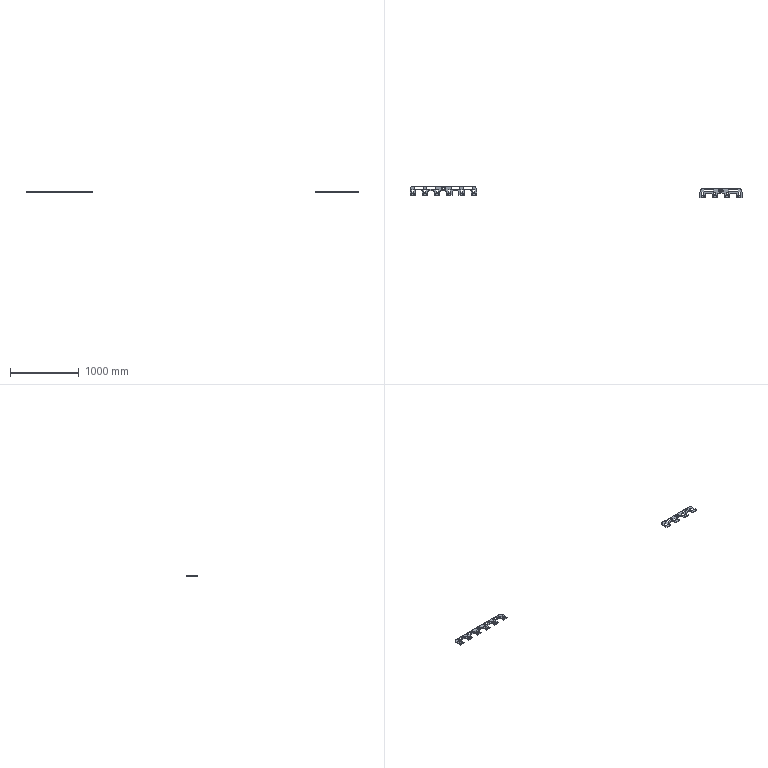NC program | NX | posted with a generic post | part box 4825 x 168.213 x 13 mm
Lines 138 to 1364 of 14244:
(ZLEVEL_PROFILE_COPY_3 , TOOL : D10)
N256 T10 M6
N258 G54
N260 G17 G0 G90 X8.032 Y52.717 S9500 M3
N262 G43 Z30. H10
N264 Z1.5
N266 G94 G1 X8.068 Y52.76 Z1.497 F1000.
N268 X10.015 Y54.925 Z1.344
N270 X12.075 Y56.985 Z1.192
N272 X14.24 Y58.932 Z1.039
N274 X16.505 Y60.763 Z0.887
N276 X18.864 Y62.471 Z0.734
N278 X21.309 Y64.053 Z0.581
N280 X23.835 Y65.503 Z0.429
N282 X26.434 Y66.817 Z0.276
N284 X29.098 Y67.992 Z0.123
N286 X31.821 Y69.025 Z-0.029
N288 X34.595 Y69.913 Z-0.182
N290 X37.412 Y70.653 Z-0.334
N292 X40.264 Y71.243 Z-0.487
N294 X43.143 Y71.682 Z-0.64
N296 X46.041 Y71.968 Z-0.792
N298 X48.95 Y72.1 Z-0.945
N300 X50. Z-1.
N302 X916.8 F3500.
N304 G2 X971.9 Y17. R55.1
N306 G1 Y-67.
N308 G2 X966.8 Y-72.1 R5.1
N310 G1 X889.
N312 G2 X883.9 Y-67. R5.1
N314 G1 Y-5.
N316 G3 X869. Y9.9 R14.9
N318 G1 X809.
N320 G3 X794.1 Y-5. R14.9
N322 G1 Y-67.
N324 G2 X789. Y-72.1 R5.1
N326 G1 X711.2
N328 G2 X706.1 Y-67. R5.1
N330 G1 Y-20.95
N332 G3 X691.2 Y-6.05 R14.9
N334 G1 X631.2
N336 G3 X616.3 Y-20.95 R14.9
N338 G1 Y-67.
N340 G2 X611.2 Y-72.1 R5.1
N342 G1 X533.4
N344 G2 X528.3 Y-67. R5.1
N346 G1 Y-20.95
N348 G3 X513.4 Y-6.05 R14.9
N350 G1 X453.4
N352 G3 X438.5 Y-20.95 R14.9
N354 G1 Y-67.
N356 G2 X433.4 Y-72.1 R5.1
N358 G1 X355.6
N360 G2 X350.5 Y-67. R5.1
N362 G1 Y-20.95
N364 G3 X335.6 Y-6.05 R14.9
N366 G1 X275.6
N368 G3 X260.7 Y-20.95 R14.9
N370 G1 Y-67.
N372 G2 X255.6 Y-72.1 R5.1
N374 G1 X177.8
N376 G2 X172.7 Y-67. R5.1
N378 G1 Y-5.
N380 G3 X157.8 Y9.9 R14.9
N382 G1 X97.8
N384 G3 X82.9 Y-5. R14.9
N386 G1 Y-67.
N388 G2 X77.8 Y-72.1 R5.1
N390 G1 X0.
N392 G2 X-5.1 Y-67. R5.1
N394 G1 Y17.
N396 G2 X50. Y72.1 R55.1
N398 G1 X107.29 Z-2.
N400 X916.8
N402 G2 X971.9 Y17. R55.1
N404 G1 Y-67.
N406 G2 X966.8 Y-72.1 R5.1
N408 G1 X889.
N410 G2 X883.9 Y-67. R5.1
N412 G1 Y-5.
N414 G3 X869. Y9.9 R14.9
N416 G1 X809.
N418 G3 X794.1 Y-5. R14.9
N420 G1 Y-67.
N422 G2 X789. Y-72.1 R5.1
N424 G1 X711.2
N426 G2 X706.1 Y-67. R5.1
N428 G1 Y-20.95
N430 G3 X691.2 Y-6.05 R14.9
N432 G1 X631.2
N434 G3 X616.3 Y-20.95 R14.9
N436 G1 Y-67.
N438 G2 X611.2 Y-72.1 R5.1
N440 G1 X533.4
N442 G2 X528.3 Y-67. R5.1
N444 G1 Y-20.95
N446 G3 X513.4 Y-6.05 R14.9
N448 G1 X453.4
N450 G3 X438.5 Y-20.95 R14.9
N452 G1 Y-67.
N454 G2 X433.4 Y-72.1 R5.1
N456 G1 X355.6
N458 G2 X350.5 Y-67. R5.1
N460 G1 Y-20.95
N462 G3 X335.6 Y-6.05 R14.9
N464 G1 X275.6
N466 G3 X260.7 Y-20.95 R14.9
N468 G1 Y-67.
N470 G2 X255.6 Y-72.1 R5.1
N472 G1 X177.8
N474 G2 X172.7 Y-67. R5.1
N476 G1 Y-5.
N478 G3 X157.8 Y9.9 R14.9
N480 G1 X97.8
N482 G3 X82.9 Y-5. R14.9
N484 G1 Y-67.
N486 G2 X77.8 Y-72.1 R5.1
N488 G1 X0.
N490 G2 X-5.1 Y-67. R5.1
N492 G1 Y17.
N494 G2 X50. Y72.1 R55.1
N496 G1 X107.29 Z-3.
N498 X916.8
N500 G2 X971.9 Y17. R55.1
N502 G1 Y-67.
N504 G2 X966.8 Y-72.1 R5.1
N506 G1 X889.
N508 G2 X883.9 Y-67. R5.1
N510 G1 Y-5.
N512 G3 X869. Y9.9 R14.9
N514 G1 X809.
N516 G3 X794.1 Y-5. R14.9
N518 G1 Y-67.
N520 G2 X789. Y-72.1 R5.1
N522 G1 X711.2
N524 G2 X706.1 Y-67. R5.1
N526 G1 Y-20.95
N528 G3 X691.2 Y-6.05 R14.9
N530 G1 X631.2
N532 G3 X616.3 Y-20.95 R14.9
N534 G1 Y-67.
N536 G2 X611.2 Y-72.1 R5.1
N538 G1 X533.4
N540 G2 X528.3 Y-67. R5.1
N542 G1 Y-20.95
N544 G3 X513.4 Y-6.05 R14.9
N546 G1 X453.4
N548 G3 X438.5 Y-20.95 R14.9
N550 G1 Y-67.
N552 G2 X433.4 Y-72.1 R5.1
N554 G1 X355.6
N556 G2 X350.5 Y-67. R5.1
N558 G1 Y-20.95
N560 G3 X335.6 Y-6.05 R14.9
N562 G1 X275.6
N564 G3 X260.7 Y-20.95 R14.9
N566 G1 Y-67.
N568 G2 X255.6 Y-72.1 R5.1
N570 G1 X177.8
N572 G2 X172.7 Y-67. R5.1
N574 G1 Y-5.
N576 G3 X157.8 Y9.9 R14.9
N578 G1 X97.8
N580 G3 X82.9 Y-5. R14.9
N582 G1 Y-67.
N584 G2 X77.8 Y-72.1 R5.1
N586 G1 X0.
N588 G2 X-5.1 Y-67. R5.1
N590 G1 Y17.
N592 G2 X50. Y72.1 R55.1
N594 G1 X95.832 Z-3.8
N596 X916.8
N598 G2 X971.9 Y17. R55.1
N600 G1 Y-67.
N602 G2 X966.8 Y-72.1 R5.1
N604 G1 X889.
N606 G2 X883.9 Y-67. R5.1
N608 G1 Y-5.
N610 G3 X869. Y9.9 R14.9
N612 G1 X809.
N614 G3 X794.1 Y-5. R14.9
N616 G1 Y-67.
N618 G2 X789. Y-72.1 R5.1
N620 G1 X711.2
N622 G2 X706.1 Y-67. R5.1
N624 G1 Y-20.95
N626 G3 X691.2 Y-6.05 R14.9
N628 G1 X631.2
N630 G3 X616.3 Y-20.95 R14.9
N632 G1 Y-67.
N634 G2 X611.2 Y-72.1 R5.1
N636 G1 X533.4
N638 G2 X528.3 Y-67. R5.1
N640 G1 Y-20.95
N642 G3 X513.4 Y-6.05 R14.9
N644 G1 X453.4
N646 G3 X438.5 Y-20.95 R14.9
N648 G1 Y-67.
N650 G2 X433.4 Y-72.1 R5.1
N652 G1 X355.6
N654 G2 X350.5 Y-67. R5.1
N656 G1 Y-20.95
N658 G3 X335.6 Y-6.05 R14.9
N660 G1 X275.6
N662 G3 X260.7 Y-20.95 R14.9
N664 G1 Y-67.
N666 G2 X255.6 Y-72.1 R5.1
N668 G1 X177.8
N670 G2 X172.7 Y-67. R5.1
N672 G1 Y-5.
N674 G3 X157.8 Y9.9 R14.9
N676 G1 X97.8
N678 G3 X82.9 Y-5. R14.9
N680 G1 Y-67.
N682 G2 X77.8 Y-72.1 R5.1
N684 G1 X0.
N686 G2 X-5.1 Y-67. R5.1
N688 G1 Y17.
N690 G2 X50. Y72.1 R55.1
N692 G1 X95.832 Z-4.6
N694 X916.8
N696 G2 X971.9 Y17. R55.1
N698 G1 Y-67.
N700 G2 X966.8 Y-72.1 R5.1
N702 G1 X889.
N704 G2 X883.9 Y-67. R5.1
N706 G1 Y-5.
N708 G3 X869. Y9.9 R14.9
N710 G1 X809.
N712 G3 X794.1 Y-5. R14.9
N714 G1 Y-67.
N716 G2 X789. Y-72.1 R5.1
N718 G1 X711.2
N720 G2 X706.1 Y-67. R5.1
N722 G1 Y-20.95
N724 G3 X691.2 Y-6.05 R14.9
N726 G1 X631.2
N728 G3 X616.3 Y-20.95 R14.9
N730 G1 Y-67.
N732 G2 X611.2 Y-72.1 R5.1
N734 G1 X533.4
N736 G2 X528.3 Y-67. R5.1
N738 G1 Y-20.95
N740 G3 X513.4 Y-6.05 R14.9
N742 G1 X453.4
N744 G3 X438.5 Y-20.95 R14.9
N746 G1 Y-67.
N748 G2 X433.4 Y-72.1 R5.1
N750 G1 X355.6
N752 G2 X350.5 Y-67. R5.1
N754 G1 Y-20.95
N756 G3 X335.6 Y-6.05 R14.9
N758 G1 X275.6
N760 G3 X260.7 Y-20.95 R14.9
N762 G1 Y-67.
N764 G2 X255.6 Y-72.1 R5.1
N766 G1 X177.8
N768 G2 X172.7 Y-67. R5.1
N770 G1 Y-5.
N772 G3 X157.8 Y9.9 R14.9
N774 G1 X97.8
N776 G3 X82.9 Y-5. R14.9
N778 G1 Y-67.
N780 G2 X77.8 Y-72.1 R5.1
N782 G1 X0.
N784 G2 X-5.1 Y-67. R5.1
N786 G1 Y17.
N788 G2 X50. Y72.1 R55.1
N790 G1 X105.858 Z-5.575
N792 X916.8
N794 G2 X971.9 Y17. R55.1
N796 G1 Y-67.
N798 G2 X966.8 Y-72.1 R5.1
N800 G1 X889.
N802 G2 X883.9 Y-67. R5.1
N804 G1 Y-5.
N806 G3 X869. Y9.9 R14.9
N808 G1 X809.
N810 G3 X794.1 Y-5. R14.9
N812 G1 Y-67.
N814 G2 X789. Y-72.1 R5.1
N816 G1 X711.2
N818 G2 X706.1 Y-67. R5.1
N820 G1 Y-20.95
N822 G3 X691.2 Y-6.05 R14.9
N824 G1 X631.2
N826 G3 X616.3 Y-20.95 R14.9
N828 G1 Y-67.
N830 G2 X611.2 Y-72.1 R5.1
N832 G1 X533.4
N834 G2 X528.3 Y-67. R5.1
N836 G1 Y-20.95
N838 G3 X513.4 Y-6.05 R14.9
N840 G1 X453.4
N842 G3 X438.5 Y-20.95 R14.9
N844 G1 Y-67.
N846 G2 X433.4 Y-72.1 R5.1
N848 G1 X355.6
N850 G2 X350.5 Y-67. R5.1
N852 G1 Y-20.95
N854 G3 X335.6 Y-6.05 R14.9
N856 G1 X275.6
N858 G3 X260.7 Y-20.95 R14.9
N860 G1 Y-67.
N862 G2 X255.6 Y-72.1 R5.1
N864 G1 X177.8
N866 G2 X172.7 Y-67. R5.1
N868 G1 Y-5.
N870 G3 X157.8 Y9.9 R14.9
N872 G1 X97.8
N874 G3 X82.9 Y-5. R14.9
N876 G1 Y-67.
N878 G2 X77.8 Y-72.1 R5.1
N880 G1 X0.
N882 G2 X-5.1 Y-67. R5.1
N884 G1 Y17.
N886 G2 X50. Y72.1 R55.1
N888 G1 X105.858 Z-6.55
N890 X916.8
N892 G2 X971.9 Y17. R55.1
N894 G1 Y-67.
N896 G2 X966.8 Y-72.1 R5.1
N898 G1 X889.
N900 G2 X883.9 Y-67. R5.1
N902 G1 Y-5.
N904 G3 X869. Y9.9 R14.9
N906 G1 X809.
N908 G3 X794.1 Y-5. R14.9
N910 G1 Y-67.
N912 G2 X789. Y-72.1 R5.1
N914 G1 X711.2
N916 G2 X706.1 Y-67. R5.1
N918 G1 Y-20.95
N920 G3 X691.2 Y-6.05 R14.9
N922 G1 X631.2
N924 G3 X616.3 Y-20.95 R14.9
N926 G1 Y-67.
N928 G2 X611.2 Y-72.1 R5.1
N930 G1 X533.4
N932 G2 X528.3 Y-67. R5.1
N934 G1 Y-20.95
N936 G3 X513.4 Y-6.05 R14.9
N938 G1 X453.4
N940 G3 X438.5 Y-20.95 R14.9
N942 G1 Y-67.
N944 G2 X433.4 Y-72.1 R5.1
N946 G1 X355.6
N948 G2 X350.5 Y-67. R5.1
N950 G1 Y-20.95
N952 G3 X335.6 Y-6.05 R14.9
N954 G1 X275.6
N956 G3 X260.7 Y-20.95 R14.9
N958 G1 Y-67.
N960 G2 X255.6 Y-72.1 R5.1
N962 G1 X177.8
N964 G2 X172.7 Y-67. R5.1
N966 G1 Y-5.
N968 G3 X157.8 Y9.9 R14.9
N970 G1 X97.8
N972 G3 X82.9 Y-5. R14.9
N974 G1 Y-67.
N976 G2 X77.8 Y-72.1 R5.1
N978 G1 X0.
N980 G2 X-5.1 Y-67. R5.1
N982 G1 Y17.
N984 G2 X50. Y72.1 R55.1
N986 G1 X105.858 Z-7.525
N988 X916.8
N990 G2 X971.9 Y17. R55.1
N992 G1 Y-67.
N994 G2 X966.8 Y-72.1 R5.1
N996 G1 X889.
N998 G2 X883.9 Y-67. R5.1
N1000 G1 Y-5.
N1002 G3 X869. Y9.9 R14.9
N1004 G1 X809.
N1006 G3 X794.1 Y-5. R14.9
N1008 G1 Y-67.
N1010 G2 X789. Y-72.1 R5.1
N1012 G1 X711.2
N1014 G2 X706.1 Y-67. R5.1
N1016 G1 Y-20.95
N1018 G3 X691.2 Y-6.05 R14.9
N1020 G1 X631.2
N1022 G3 X616.3 Y-20.95 R14.9
N1024 G1 Y-67.
N1026 G2 X611.2 Y-72.1 R5.1
N1028 G1 X533.4
N1030 G2 X528.3 Y-67. R5.1
N1032 G1 Y-20.95
N1034 G3 X513.4 Y-6.05 R14.9
N1036 G1 X453.4
N1038 G3 X438.5 Y-20.95 R14.9
N1040 G1 Y-67.
N1042 G2 X433.4 Y-72.1 R5.1
N1044 G1 X355.6
N1046 G2 X350.5 Y-67. R5.1
N1048 G1 Y-20.95
N1050 G3 X335.6 Y-6.05 R14.9
N1052 G1 X275.6
N1054 G3 X260.7 Y-20.95 R14.9
N1056 G1 Y-67.
N1058 G2 X255.6 Y-72.1 R5.1
N1060 G1 X177.8
N1062 G2 X172.7 Y-67. R5.1
N1064 G1 Y-5.
N1066 G3 X157.8 Y9.9 R14.9
N1068 G1 X97.8
N1070 G3 X82.9 Y-5. R14.9
N1072 G1 Y-67.
N1074 G2 X77.8 Y-72.1 R5.1
N1076 G1 X0.
N1078 G2 X-5.1 Y-67. R5.1
N1080 G1 Y17.
N1082 G2 X50. Y72.1 R55.1
N1084 G1 X105.858 Z-8.5
N1086 X916.8
N1088 G2 X971.9 Y17. R55.1
N1090 G1 Y-67.
N1092 G2 X966.8 Y-72.1 R5.1
N1094 G1 X889.
N1096 G2 X883.9 Y-67. R5.1
N1098 G1 Y-5.
N1100 G3 X869. Y9.9 R14.9
N1102 G1 X809.
N1104 G3 X794.1 Y-5. R14.9
N1106 G1 Y-67.
N1108 G2 X789. Y-72.1 R5.1
N1110 G1 X711.2
N1112 G2 X706.1 Y-67. R5.1
N1114 G1 Y-20.95
N1116 G3 X691.2 Y-6.05 R14.9
N1118 G1 X631.2
N1120 G3 X616.3 Y-20.95 R14.9
N1122 G1 Y-67.
N1124 G2 X611.2 Y-72.1 R5.1
N1126 G1 X533.4
N1128 G2 X528.3 Y-67. R5.1
N1130 G1 Y-20.95
N1132 G3 X513.4 Y-6.05 R14.9
N1134 G1 X453.4
N1136 G3 X438.5 Y-20.95 R14.9
N1138 G1 Y-67.
N1140 G2 X433.4 Y-72.1 R5.1
N1142 G1 X355.6
N1144 G2 X350.5 Y-67. R5.1
N1146 G1 Y-20.95
N1148 G3 X335.6 Y-6.05 R14.9
N1150 G1 X275.6
N1152 G3 X260.7 Y-20.95 R14.9
N1154 G1 Y-67.
N1156 G2 X255.6 Y-72.1 R5.1
N1158 G1 X177.8
N1160 G2 X172.7 Y-67. R5.1
N1162 G1 Y-5.
N1164 G3 X157.8 Y9.9 R14.9
N1166 G1 X97.8
N1168 G3 X82.9 Y-5. R14.9
N1170 G1 Y-67.
N1172 G2 X77.8 Y-72.1 R5.1
N1174 G1 X0.
N1176 G2 X-5.1 Y-67. R5.1
N1178 G1 Y17.
N1180 G2 X50. Y72.1 R55.1
N1182 G1 X105.858 Z-9.475
N1184 X916.8
N1186 G2 X971.9 Y17. R55.1
N1188 G1 Y-67.
N1190 G2 X966.8 Y-72.1 R5.1
N1192 G1 X889.
N1194 G2 X883.9 Y-67. R5.1
N1196 G1 Y-5.
N1198 G3 X869. Y9.9 R14.9
N1200 G1 X809.
N1202 G3 X794.1 Y-5. R14.9
N1204 G1 Y-67.
N1206 G2 X789. Y-72.1 R5.1
N1208 G1 X711.2
N1210 G2 X706.1 Y-67. R5.1
N1212 G1 Y-20.95
N1214 G3 X691.2 Y-6.05 R14.9
N1216 G1 X631.2
N1218 G3 X616.3 Y-20.95 R14.9
N1220 G1 Y-67.
N1222 G2 X611.2 Y-72.1 R5.1
N1224 G1 X533.4
N1226 G2 X528.3 Y-67. R5.1
N1228 G1 Y-20.95
N1230 G3 X513.4 Y-6.05 R14.9
N1232 G1 X453.4
N1234 G3 X438.5 Y-20.95 R14.9
N1236 G1 Y-67.
N1238 G2 X433.4 Y-72.1 R5.1
N1240 G1 X355.6
N1242 G2 X350.5 Y-67. R5.1
N1244 G1 Y-20.95
N1246 G3 X335.6 Y-6.05 R14.9
N1248 G1 X275.6
N1250 G3 X260.7 Y-20.95 R14.9
N1252 G1 Y-67.
N1254 G2 X255.6 Y-72.1 R5.1
N1256 G1 X177.8
N1258 G2 X172.7 Y-67. R5.1
N1260 G1 Y-5.
N1262 G3 X157.8 Y9.9 R14.9
N1264 G1 X97.8
N1266 G3 X82.9 Y-5. R14.9
N1268 G1 Y-67.
N1270 G2 X77.8 Y-72.1 R5.1
N1272 G1 X0.
N1274 G2 X-5.1 Y-67. R5.1
N1276 G1 Y17.
N1278 G2 X50. Y72.1 R55.1
N1280 G1 X105.858 Z-10.45
N1282 X916.8
N1284 G2 X971.9 Y17. R55.1
N1286 G1 Y-67.
N1288 G2 X966.8 Y-72.1 R5.1
N1290 G1 X889.
N1292 G2 X883.9 Y-67. R5.1
N1294 G1 Y-5.
N1296 G3 X869. Y9.9 R14.9
N1298 G1 X809.
N1300 G3 X794.1 Y-5. R14.9
N1302 G1 Y-67.
N1304 G2 X789. Y-72.1 R5.1
N1306 G1 X711.2
N1308 G2 X706.1 Y-67. R5.1
N1310 G1 Y-20.95
N1312 G3 X691.2 Y-6.05 R14.9
N1314 G1 X631.2
N1316 G3 X616.3 Y-20.95 R14.9
N1318 G1 Y-67.
N1320 G2 X611.2 Y-72.1 R5.1
N1322 G1 X533.4
N1324 G2 X528.3 Y-67. R5.1
N1326 G1 Y-20.95
N1328 G3 X513.4 Y-6.05 R14.9
N1330 G1 X453.4
N1332 G3 X438.5 Y-20.95 R14.9
N1334 G1 Y-67.
N1336 G2 X433.4 Y-72.1 R5.1
N1338 G1 X355.6
N1340 G2 X350.5 Y-67. R5.1
N1342 G1 Y-20.95
N1344 G3 X335.6 Y-6.05 R14.9
N1346 G1 X275.6
N1348 G3 X260.7 Y-20.95 R14.9
N1350 G1 Y-67.
N1352 G2 X255.6 Y-72.1 R5.1
N1354 G1 X177.8
N1356 G2 X172.7 Y-67. R5.1
N1358 G1 Y-5.
N1360 G3 X157.8 Y9.9 R14.9
N1362 G1 X97.8
N1364 G3 X82.9 Y-5. R14.9
N1366 G1 Y-67.
N1368 G2 X77.8 Y-72.1 R5.1
N1370 G1 X0.
N1372 G2 X-5.1 Y-67. R5.1
N1374 G1 Y17.
N1376 G2 X50. Y72.1 R55.1
N1378 G1 X105.858 Z-11.425
N1380 X916.8
N1382 G2 X971.9 Y17. R55.1
N1384 G1 Y-67.
N1386 G2 X966.8 Y-72.1 R5.1
N1388 G1 X889.
N1390 G2 X883.9 Y-67. R5.1
N1392 G1 Y-5.
N1394 G3 X869. Y9.9 R14.9
N1396 G1 X809.
N1398 G3 X794.1 Y-5. R14.9
N1400 G1 Y-67.
N1402 G2 X789. Y-72.1 R5.1
N1404 G1 X711.2
N1406 G2 X706.1 Y-67. R5.1
N1408 G1 Y-20.95
N1410 G3 X691.2 Y-6.05 R14.9
N1412 G1 X631.2
N1414 G3 X616.3 Y-20.95 R14.9
N1416 G1 Y-67.
N1418 G2 X611.2 Y-72.1 R5.1
N1420 G1 X533.4
N1422 G2 X528.3 Y-67. R5.1
N1424 G1 Y-20.95
N1426 G3 X513.4 Y-6.05 R14.9
N1428 G1 X453.4
N1430 G3 X438.5 Y-20.95 R14.9
N1432 G1 Y-67.
N1434 G2 X433.4 Y-72.1 R5.1
N1436 G1 X355.6
N1438 G2 X350.5 Y-67. R5.1
N1440 G1 Y-20.95
N1442 G3 X335.6 Y-6.05 R14.9
N1444 G1 X275.6
N1446 G3 X260.7 Y-20.95 R14.9
N1448 G1 Y-67.
N1450 G2 X255.6 Y-72.1 R5.1
N1452 G1 X177.8
N1454 G2 X172.7 Y-67. R5.1
N1456 G1 Y-5.
N1458 G3 X157.8 Y9.9 R14.9
N1460 G1 X97.8
N1462 G3 X82.9 Y-5. R14.9
N1464 G1 Y-67.
N1466 G2 X77.8 Y-72.1 R5.1
N1468 G1 X0.
N1470 G2 X-5.1 Y-67. R5.1
N1472 G1 Y17.
N1474 G2 X50. Y72.1 R55.1
N1476 G1 X105.858 Z-12.4
N1478 X916.8
N1480 G2 X971.9 Y17. R55.1
N1482 G1 Y-67.
N1484 G2 X966.8 Y-72.1 R5.1
N1486 G1 X889.
N1488 G2 X883.9 Y-67. R5.1
N1490 G1 Y-5.
N1492 G3 X869. Y9.9 R14.9
N1494 G1 X809.
N1496 G3 X794.1 Y-5. R14.9
N1498 G1 Y-67.
N1500 G2 X789. Y-72.1 R5.1
N1502 G1 X711.2
N1504 G2 X706.1 Y-67. R5.1
N1506 G1 Y-20.95
N1508 G3 X691.2 Y-6.05 R14.9
N1510 G1 X631.2
N1512 G3 X616.3 Y-20.95 R14.9
N1514 G1 Y-67.
N1516 G2 X611.2 Y-72.1 R5.1
N1518 G1 X533.4
N1520 G2 X528.3 Y-67. R5.1
N1522 G1 Y-20.95
N1524 G3 X513.4 Y-6.05 R14.9
N1526 G1 X453.4
N1528 G3 X438.5 Y-20.95 R14.9
N1530 G1 Y-67.
N1532 G2 X433.4 Y-72.1 R5.1
N1534 G1 X355.6
N1536 G2 X350.5 Y-67. R5.1
N1538 G1 Y-20.95
N1540 G3 X335.6 Y-6.05 R14.9
N1542 G1 X275.6
N1544 G3 X260.7 Y-20.95 R14.9
N1546 G1 Y-67.
N1548 G2 X255.6 Y-72.1 R5.1
N1550 G1 X177.8
N1552 G2 X172.7 Y-67. R5.1
N1554 G1 Y-5.
N1556 G3 X157.8 Y9.9 R14.9
N1558 G1 X97.8
N1560 G3 X82.9 Y-5. R14.9
N1562 G1 Y-67.
N1564 G2 X77.8 Y-72.1 R5.1
N1566 G1 X0.
N1568 G2 X-5.1 Y-67. R5.1
N1570 G1 Y17.
N1572 G2 X50. Y72.1 R55.1
N1574 G1 X105.858
N1576 Z-10.9
N1578 G0 Z30.
(ZLEVEL_PROFILE_COPY_2_COPY , TOOL : D10)
N1580 X353.303 Y51.9
N1582 Z1.5
N1584 G1 X305.6 Z-1. F1000.
N1586 X246.814 F3500.
N1588 X246.8 Y51.902
N1590 Y30.1
N1592 X364.4
N1594 Y51.902
N1596 X364.365 Y51.9
N1598 X305.6
N1600 X248.31 Z-2.
N1602 X246.814
N1604 X246.8 Y51.902
N1606 Y30.1
N1608 X364.4
N1610 Y51.902
N1612 X364.365 Y51.9
N1614 X305.6
N1616 X248.31 Z-3.
N1618 X246.814
N1620 X246.8 Y51.902
N1622 Y30.1
N1624 X364.4
N1626 Y51.902
N1628 X364.365 Y51.9
N1630 X305.6
N1632 X259.768 Z-3.8
N1634 X246.814
N1636 X246.8 Y51.902
N1638 Y30.1
N1640 X364.4
N1642 Y51.902
N1644 X364.365 Y51.9
N1646 X305.6
N1648 X259.768 Z-4.6
N1650 X246.814
N1652 X246.8 Y51.902
N1654 Y30.1
N1656 X364.4
N1658 Y51.902
N1660 X364.365 Y51.9
N1662 X305.6
N1664 X252.766 Z-5.522
N1666 X246.814
N1668 X246.8 Y51.902
N1670 Y30.1
N1672 X364.4
N1674 Y51.902
N1676 X364.365 Y51.9
N1678 X305.6
N1680 X252.766 Z-6.444
N1682 X246.814
N1684 X246.8 Y51.902
N1686 Y30.1
N1688 X364.4
N1690 Y51.902
N1692 X364.365 Y51.9
N1694 X305.6
N1696 X252.766 Z-7.367
N1698 X246.814
N1700 X246.8 Y51.902
N1702 Y30.1
N1704 X364.4
N1706 Y51.902
N1708 X364.365 Y51.9
N1710 X305.6
N1712 X252.766 Z-8.289
N1714 X246.811
N1716 X246.8 Y51.902
N1718 Y30.1
N1720 X364.4
N1722 Y51.902
N1724 X364.365 Y51.9
N1726 X305.6
N1728 X252.766 Z-9.211
N1730 X246.811
N1732 X246.8 Y51.902
N1734 Y30.1
N1736 X364.4
N1738 Y51.902
N1740 X364.365 Y51.9
N1742 X305.6
N1744 X252.766 Z-10.133
N1746 X246.811
N1748 X246.8 Y51.902
N1750 Y30.1
N1752 X364.4
N1754 Y51.902
N1756 X364.365 Y51.9
N1758 X305.6
N1760 X252.766 Z-11.056
N1762 X246.811
N1764 X246.8 Y51.902
N1766 Y30.1
N1768 X364.4
N1770 Y51.902
N1772 X364.365 Y51.9
N1774 X305.6
N1776 X252.766 Z-11.978
N1778 X246.811
N1780 X246.8 Y51.902
N1782 Y30.1
N1784 X364.4
N1786 Y51.902
N1788 X364.365 Y51.9
N1790 X305.6
N1792 X252.766 Z-12.9
N1794 X246.811
N1796 X246.8 Y51.902
N1798 Y30.1
N1800 X364.4
N1802 Y51.902
N1804 X364.365 Y51.9
N1806 X252.766
N1808 Z-11.4
N1810 G0 Z30.
N1812 X175.503
N1814 Z1.5
N1816 G1 X127.8 Z-1. F1000.
N1818 X69.038 F3500.
N1820 X69. Y51.902
N1822 Y30.1
N1824 X186.6
N1826 Y51.902
N1828 X186.561 Y51.9
N1830 X127.8
N1832 X70.51 Z-2.
N1834 X69.038
N1836 X69. Y51.902
N1838 Y30.1
N1840 X186.6
N1842 Y51.902
N1844 X186.561 Y51.9
N1846 X127.8
N1848 X70.51 Z-3.
N1850 X69.038
N1852 X69. Y51.902
N1854 Y30.1
N1856 X186.6
N1858 Y51.902
N1860 X186.561 Y51.9
N1862 X127.8
N1864 X81.968 Z-3.8
N1866 X69.038
N1868 X69. Y51.902
N1870 Y30.1
N1872 X186.6
N1874 Y51.902
N1876 X186.561 Y51.9
N1878 X127.8
N1880 X81.968 Z-4.6
N1882 X69.038
N1884 X69. Y51.902
N1886 Y30.1
N1888 X186.6
N1890 Y51.902
N1892 X186.561 Y51.9
N1894 X127.8
N1896 X74.966 Z-5.522
N1898 X69.038
N1900 X69. Y51.902
N1902 Y30.1
N1904 X186.6
N1906 Y51.902
N1908 X186.561 Y51.9
N1910 X127.8
N1912 X74.966 Z-6.444
N1914 X69.038
N1916 X69. Y51.902
N1918 Y30.1
N1920 X186.6
N1922 Y51.902
N1924 X186.561 Y51.9
N1926 X127.8
N1928 X74.966 Z-7.367
N1930 X69.038
N1932 X69. Y51.902
N1934 Y30.1
N1936 X186.6
N1938 Y51.902
N1940 X186.561 Y51.9
N1942 X127.8
N1944 X74.966 Z-8.289
N1946 X69.038
N1948 X69. Y51.902
N1950 Y30.1
N1952 X186.6
N1954 Y51.902
N1956 X186.561 Y51.9
N1958 X127.8
N1960 X74.966 Z-9.211
N1962 X69.038
N1964 X69. Y51.902
N1966 Y30.1
N1968 X186.6
N1970 Y51.902
N1972 X186.561 Y51.9
N1974 X127.8
N1976 X74.966 Z-10.133
N1978 X69.038
N1980 X69. Y51.902
N1982 Y30.1
N1984 X186.6
N1986 Y51.902
N1988 X186.561 Y51.9
N1990 X127.8
N1992 X74.966 Z-11.056
N1994 X69.038
N1996 X69. Y51.902
N1998 Y30.1
N2000 X186.6
N2002 Y51.902
N2004 X186.561 Y51.9
N2006 X127.8
N2008 X74.966 Z-11.978
N2010 X69.038
N2012 X69. Y51.902
N2014 Y30.1
N2016 X186.6
N2018 Y51.902
N2020 X186.561 Y51.9
N2022 X127.8
N2024 X74.966 Z-12.9
N2026 X69.038
N2028 X69. Y51.902
N2030 Y30.1
N2032 X186.6
N2034 Y51.902
N2036 X186.561 Y51.9
N2038 X74.966
N2040 Z-11.4
N2042 G0 Z30.
N2044 X404.4 Y-2.099
N2046 Z1.5
N2048 G1 Y10.902 Z0.819 F1000.
N2050 X404.353 Y10.9 Z0.816
N2052 X384.649 Z-0.216
N2054 X384.6 Y10.903 Z-0.219
N2056 Y-3.999 Z-1.
N2058 Y-18.9 F3500.
N2060 X404.4
N2062 Y10.902
N2064 X404.353 Y10.9
N2066 X384.649
N2068 X384.6 Y10.903
N2070 Y-3.999
N2072 Y-18.9 Z-1.26
N2074 X404.4 Z-1.606
N2076 Y3.689 Z-2.
N2078 Y10.902
N2080 X404.353 Y10.9
N2082 X384.649
N2084 X384.6 Y10.903
N2086 Y-3.999
N2088 Y-18.9 Z-2.26
N2090 X404.4 Z-2.606
N2092 Y3.689 Z-3.
N2094 Y10.902
N2096 X404.353 Y10.9
N2098 X384.649
N2100 X384.6 Y10.903
N2102 Y-3.999
N2104 Y-18.9 Z-3.26
N2106 X404.184 Z-3.602
N2108 X404.4 Y-18.894 Z-3.606
N2110 Y-7.769 Z-3.8
N2112 Y10.902
N2114 X404.353 Y10.9
N2116 X384.649
N2118 X384.6 Y10.903
N2120 Y-3.999
N2122 Y-18.9 Z-4.06
N2124 X404.184 Z-4.402
N2126 X404.4 Y-18.894 Z-4.406
N2128 Y-7.769 Z-4.6
N2130 Y10.902
N2132 X404.353 Y10.9
N2134 X384.649
N2136 X384.6 Y10.903
N2138 Y-3.999
N2140 Y-18.9 Z-4.86
N2142 X404.4 Z-5.206
N2144 Y-0.767 Z-5.522
N2146 Y10.902
N2148 X404.353 Y10.9
N2150 X384.649
N2152 X384.6 Y10.903
N2154 Y-3.999
N2156 Y-18.9 Z-5.782
N2158 X404.4 Z-6.128
N2160 Y-0.767 Z-6.444
N2162 Y10.902
N2164 X404.353 Y10.9
N2166 X384.649
N2168 X384.6 Y10.903
N2170 Y-3.999
N2172 Y-18.9 Z-6.705
N2174 X404.4 Z-7.05
N2176 Y-0.767 Z-7.367
N2178 Y10.902
N2180 X404.353 Y10.9
N2182 X384.649
N2184 X384.6 Y10.903
N2186 Y-3.999
N2188 Y-18.9 Z-7.627
N2190 X404.4 Z-7.972
N2192 Y-0.767 Z-8.289
N2194 Y10.902
N2196 X404.353 Y10.9
N2198 X384.649
N2200 X384.6 Y10.903
N2202 Y-3.999
N2204 Y-18.9 Z-8.549
N2206 X404.4 Z-8.895
N2208 Y-0.767 Z-9.211
N2210 Y10.902
N2212 X404.353 Y10.9
N2214 X384.649
N2216 X384.6 Y10.903
N2218 Y-3.999
N2220 Y-18.9 Z-9.471
N2222 X404.4 Z-9.817
N2224 Y-0.767 Z-10.133
N2226 Y10.902
N2228 X404.353 Y10.9
N2230 X384.649
N2232 X384.6 Y10.903
N2234 Y-3.999
N2236 Y-18.9 Z-10.393
N2238 X404.4 Z-10.739
N2240 Y-0.767 Z-11.056
N2242 Y10.902
N2244 X404.353 Y10.9
N2246 X384.649
N2248 X384.6 Y10.903
N2250 Y-3.999
N2252 Y-18.9 Z-11.316
N2254 X404.4 Z-11.661
N2256 Y-0.767 Z-11.978
N2258 Y10.902
N2260 X404.353 Y10.9
N2262 X384.649
N2264 X384.6 Y10.903
N2266 Y-3.999
N2268 Y-18.9 Z-12.238
N2270 X404.4 Z-12.583
N2272 Y-0.767 Z-12.9
N2274 Y10.902
N2276 X404.353 Y10.9
N2278 X384.649
N2280 X384.6 Y10.903
N2282 Y-18.9
N2284 X404.4
N2286 Y-0.767
N2288 Z-11.4
N2290 G0 Z30.
N2292 X206.8 Y-5.898
N2294 Z1.5
N2296 G1 Y-18.9 Z0.819 F1000.
N2298 X226.6 Z-0.219
N2300 Y-3.999 Z-1.
N2302 Y10.902 F3500.
N2304 X226.546 Y10.9
N2306 X206.841
N2308 X206.8 Y10.902
N2310 Y-18.9
N2312 X226.6
N2314 Y-3.999
N2316 Y10.656 Z-1.256
N2318 Y10.9 Z-1.26
N2320 X226.401 Z-1.264
N2322 X206.86 Z-1.605
N2324 X206.8 Z-1.606
N2326 Y10.518 Z-1.612
N2328 Y-11.687 Z-2.
N2330 Y-18.9
N2332 X226.6
N2334 Y-3.999
N2336 Y10.656 Z-2.256
N2338 Y10.9 Z-2.26
N2340 X226.401 Z-2.264
N2342 X206.86 Z-2.605
N2344 X206.8 Z-2.606
N2346 Y10.518 Z-2.612
N2348 Y-11.687 Z-3.
N2350 Y-18.9
N2352 X226.6
N2354 Y-3.999
N2356 Y10.685 Z-3.256
N2358 Y10.9 Z-3.26
N2360 X226.372 Z-3.264
N2362 X207.238 Z-3.598
N2364 X207.017 Z-3.602
N2366 X206.8 Y10.895 Z-3.606
N2368 Y-0.229 Z-3.8
N2370 Y-18.9
N2372 X226.6
N2374 Y-3.999
N2376 Y10.685 Z-4.056
N2378 Y10.9 Z-4.06
N2380 X226.372 Z-4.064
N2382 X207.238 Z-4.398
N2384 X207.017 Z-4.402
N2386 X206.8 Y10.895 Z-4.406
N2388 Y-0.229 Z-4.6
N2390 Y-18.9
N2392 X226.6
N2394 Y-3.999
N2396 Y10.652 Z-4.856
N2398 Y10.9 Z-4.86
N2400 X226.405 Z-4.863
N2402 X206.87 Z-5.204
N2404 X206.8 Z-5.206
N2406 Y10.528 Z-5.212
N2408 Y-7.231 Z-5.522
N2410 Y-18.9
N2412 X226.6
N2414 Y-3.999
N2416 Y10.652 Z-5.778
N2418 Y10.9 Z-5.782
N2420 X226.405 Z-5.786
N2422 X206.87 Z-6.127
N2424 X206.8 Z-6.128
N2426 Y10.528 Z-6.134
N2428 Y-7.231 Z-6.444
N2430 Y-18.9
N2432 X226.6
N2434 Y-3.999
N2436 Y10.652 Z-6.7
N2438 Y10.9 Z-6.705
N2440 X226.405 Z-6.708
N2442 X206.87 Z-7.049
N2444 X206.8 Z-7.05
N2446 Y10.528 Z-7.057
N2448 Y-7.231 Z-7.367
N2450 Y-18.9
N2452 X226.6
N2454 Y-3.999
N2456 Y10.652 Z-7.622
N2458 Y10.9 Z-7.627
N2460 X226.405 Z-7.63
N2462 X206.87 Z-7.971
N2464 X206.8 Z-7.972
N2466 Y10.528 Z-7.979
N2468 Y-7.231 Z-8.289
N2470 Y-18.9
N2472 X226.6
N2474 Y-3.999
N2476 Y10.652 Z-8.545
N2478 Y10.9 Z-8.549
N2480 X226.405 Z-8.552
N2482 X206.87 Z-8.893
N2484 X206.8 Z-8.895
N2486 Y10.528 Z-8.901
N2488 Y-7.231 Z-9.211
N2490 Y-18.9
N2492 X226.6
N2494 Y-3.999
N2496 Y10.652 Z-9.467
N2498 Y10.9 Z-9.471
N2500 X226.405 Z-9.475
N2502 X206.87 Z-9.816
N2504 X206.8 Z-9.817
N2506 Y10.528 Z-9.823
N2508 Y-7.231 Z-10.133
N2510 Y-18.9
N2512 X226.6
N2514 Y-3.999
N2516 Y10.652 Z-10.389
N2518 Y10.9 Z-10.393
N2520 X226.405 Z-10.397
N2522 X206.87 Z-10.738
N2524 X206.8 Z-10.739
N2526 Y10.528 Z-10.746
N2528 Y-7.231 Z-11.056
N2530 Y-18.9
N2532 X226.6
N2534 Y-3.999
N2536 Y10.652 Z-11.311
N2538 Y10.9 Z-11.316
N2540 X226.405 Z-11.319
N2542 X206.87 Z-11.66
N2544 X206.8 Z-11.661
N2546 Y10.528 Z-11.668
N2548 Y-7.231 Z-11.978
N2550 Y-18.9
N2552 X226.6
N2554 Y-3.999
N2556 Y10.652 Z-12.234
N2558 Y10.9 Z-12.238
N2560 X226.405 Z-12.241
N2562 X206.87 Z-12.582
N2564 X206.8 Z-12.583
N2566 Y10.528 Z-12.59
N2568 Y-7.231 Z-12.9
N2570 Y-18.9
N2572 X226.6
N2574 Y10.901
N2576 X226.546 Y10.9
N2578 X206.841
N2580 X206.8 Y10.902
N2582 Y-7.231
N2584 Z-11.4
N2586 G0 Z30.
N2588 X48.8 Y-2.099
N2590 Z1.5
N2592 G1 Y10.902 Z0.819 F1000.
N2594 X48.763 Y10.9 Z0.817
N2596 X29.035 Z-0.217
N2598 X29. Y10.902 Z-0.219
N2600 Y-3.999 Z-1.
N2602 Y-18.9 F3500.
N2604 X48.8
N2606 Y10.902
N2608 X48.763 Y10.9
N2610 X29.035
N2612 X29. Y10.902
N2614 Y-3.999
N2616 Y-18.9 Z-1.26
N2618 X48.8 Z-1.606
N2620 Y3.689 Z-2.
N2622 Y10.902
N2624 X48.763 Y10.9
N2626 X29.035
N2628 X29. Y10.902
N2630 Y-3.999
N2632 Y-18.9 Z-2.26
N2634 X48.8 Z-2.606
N2636 Y3.689 Z-3.
N2638 Y10.902
N2640 X48.763 Y10.9
N2642 X29.035
N2644 X29. Y10.902
N2646 Y-3.999
N2648 Y-18.9 Z-3.26
N2650 X48.584 Z-3.602
N2652 X48.8 Y-18.893 Z-3.606
N2654 Y-7.769 Z-3.8
N2656 Y10.902
N2658 X48.763 Y10.9
N2660 X29.035
N2662 X29. Y10.902
N2664 Y-3.999
N2666 Y-18.9 Z-4.06
N2668 X48.584 Z-4.402
N2670 X48.8 Y-18.893 Z-4.406
N2672 Y-7.769 Z-4.6
N2674 Y10.902
N2676 X48.763 Y10.9
N2678 X29.035
N2680 X29. Y10.902
N2682 Y-3.999
N2684 Y-18.9 Z-4.86
N2686 X48.8 Z-5.206
N2688 Y-0.767 Z-5.522
N2690 Y10.902
N2692 X48.763 Y10.9
N2694 X29.035
N2696 X29. Y10.902